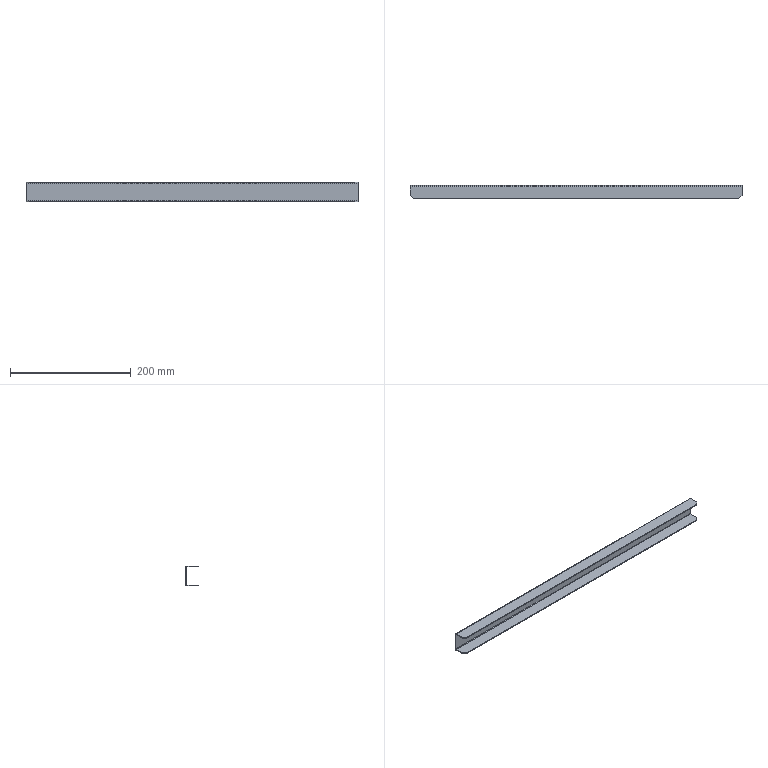Part | STEP file | b-019 | 1 solid | 26 faces | box 550 x 21.5 x 33 mm | volume 59097 mm3 | plane 22 | cylinder 4 | commonest cylinder face diameters 1.473 x2 4.473 x2